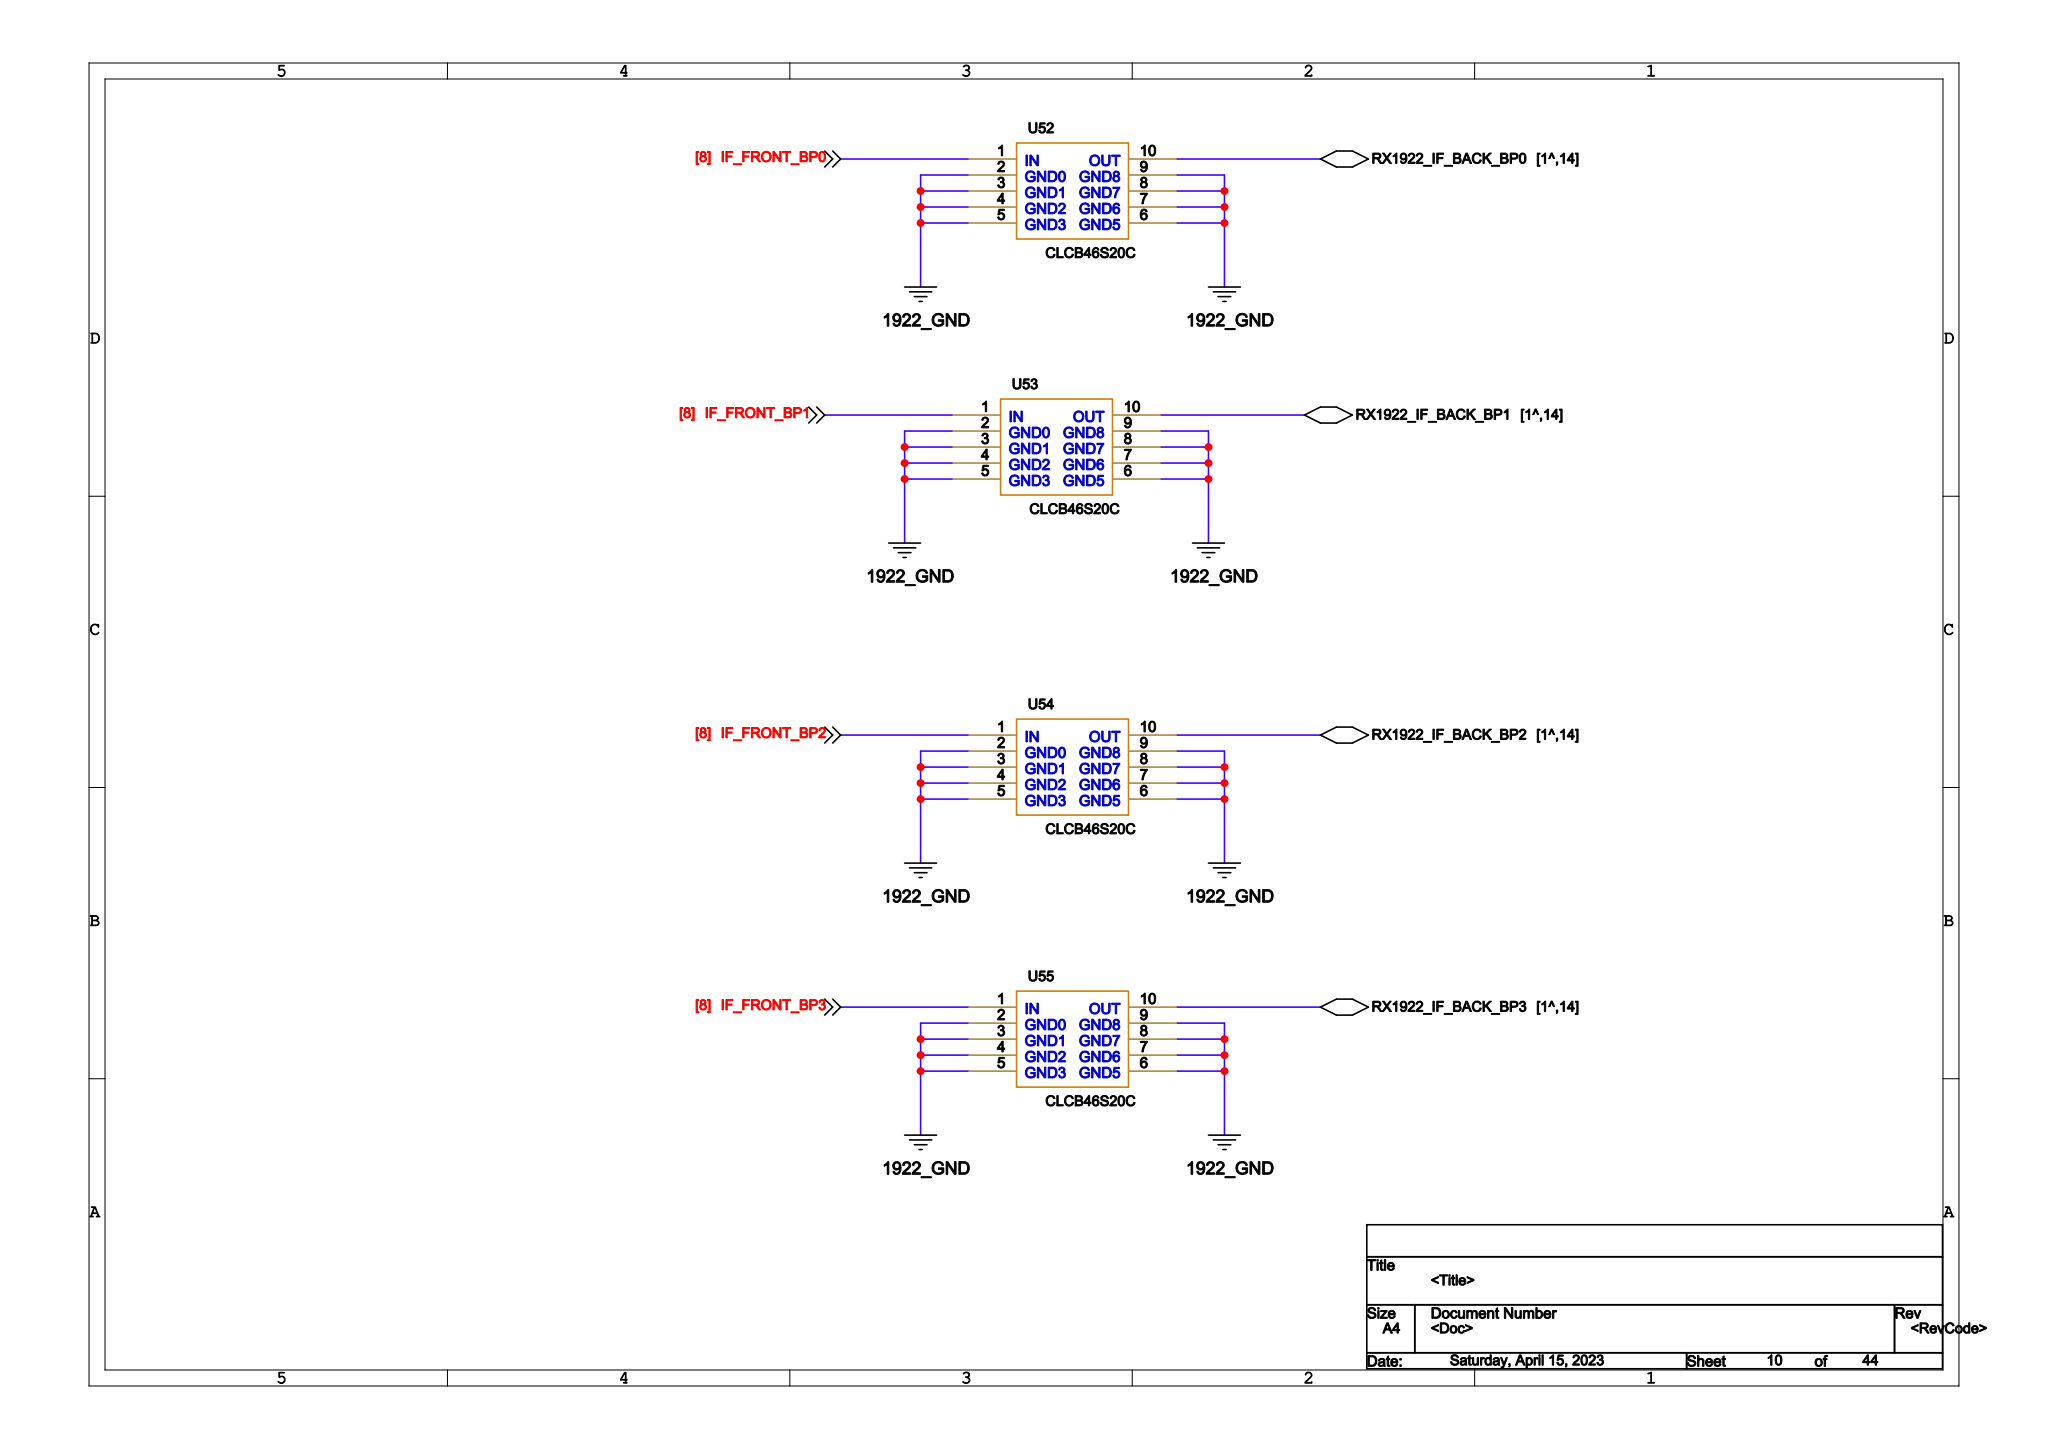Circuit board | Cadence Allegro | 1034 parts | 912 nets | one sheet of the schematic
Parts on this sheet (reference | value | footprint):
U52 | CLCB46S20C | CLCB46S20C
U53 | CLCB46S20C | CLCB46S20C
U54 | CLCB46S20C | CLCB46S20C
U55 | CLCB46S20C | CLCB46S20C
Nets of these parts (net: part-pin ...):
IF_FRONT_BP0_D1: U52-1
IF_FRONT_BP1_D1: U53-1
IF_FRONT_BP2_D1: U54-1
IF_FRONT_BP3_D1: U55-1
1922_GND: U52-2 U52-3 U52-4 U52-5 U52-6 U52-7 U52-8 U52-9 U53-2 U53-3 U53-4 U53-5 U53-6 U53-7 U53-8 U53-9 U54-2 U54-3 U54-4 U54-5 U54-6 U54-7 U54-8 U54-9 U55-2 U55-3 U55-4 U55-5 U55-6 U55-7 U55-8 U55-9
N186037: U53-10
N186039: U54-10
N186035: U52-10
N186041: U55-10